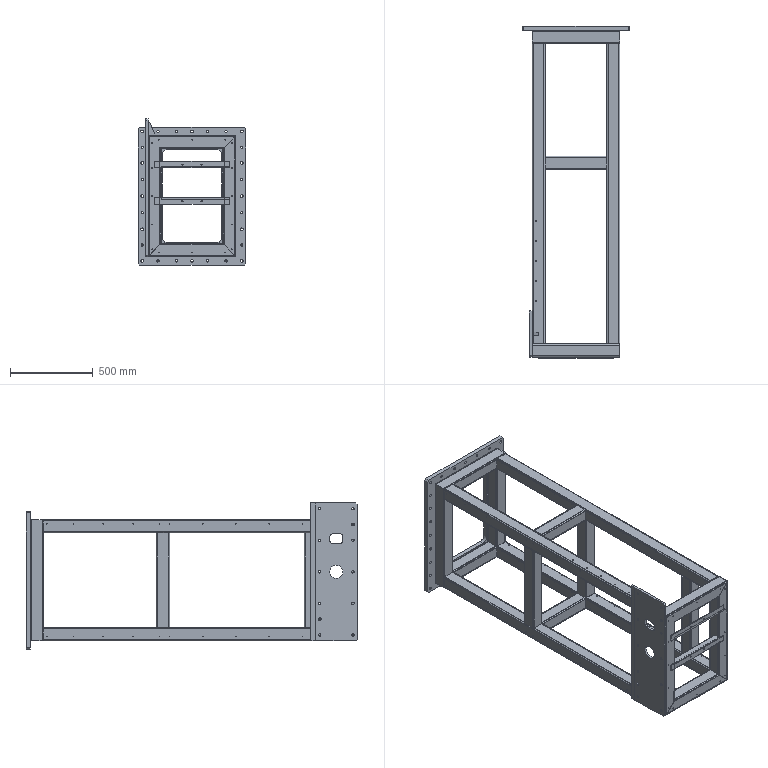Part | SolidWorks | features HoleWzd 24, WeldCornerFeat 14, ICE 8, WeldMemberFeat 4, Chamfer 2, Fillet 2, 3DProfileFeature 1, WeldmentFeature 1 | 19 solids | 714 faces | box 650 x 2000 x 880 mm | volume 28196687 mm3 | cylinder 490 | plane 220 | cone 4 | commonest cylinder face diameters 3.3 x228 16 x72 8 x68 14 x54 16.5 x24 5 x20